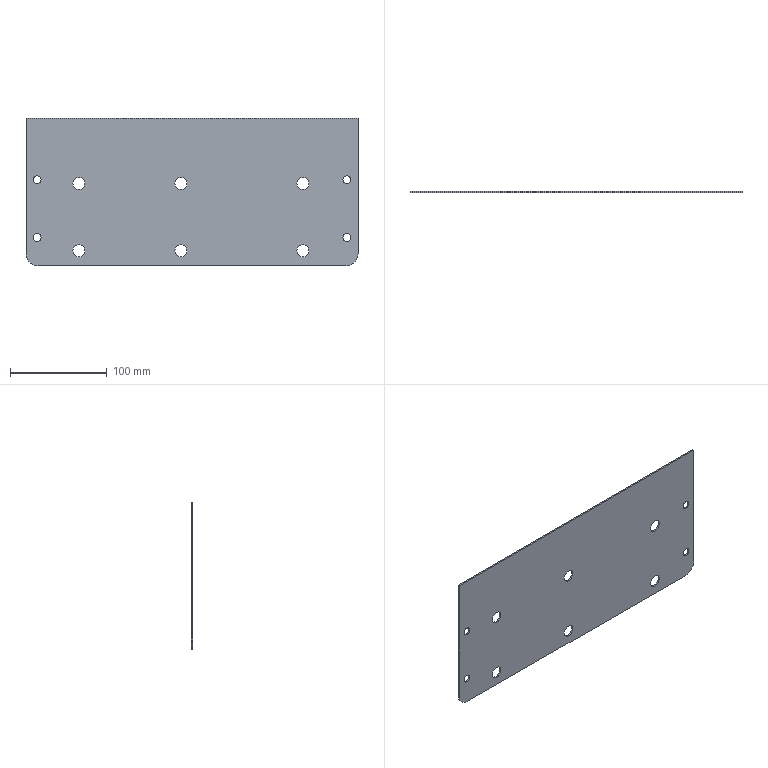Part | NX | features BREP 1 | 1 solid | 28 faces | box 342.9 x 1.499 x 152.4 mm | volume 76805 mm3 | cylinder 22 | plane 6 | commonest cylinder face diameters 12.446 x12 8.128 x8 25.4 x2
STEP:
#1=CARTESIAN_POINT('',(158.75,0.,-152.4));
#2=VERTEX_POINT('',#1);
#3=CARTESIAN_POINT('',(-158.75,0.,-152.4));
#4=VERTEX_POINT('',#3);
#5=CARTESIAN_POINT('',(158.75,0.,-152.4));
#6=DIRECTION('',(-1.,0.,0.));
#7=VECTOR('',#6,1000.);
#8=LINE('',#5,#7);
#9=EDGE_CURVE('',#2,#4,#8,.T.);
#10=ORIENTED_EDGE('',*,*,#9,.T.);
#11=CARTESIAN_POINT('',(-171.45,0.,-139.7));
#12=VERTEX_POINT('',#11);
#13=CARTESIAN_POINT('',(-158.75,0.,-139.7));
#14=DIRECTION('',(0.,1.,0.));
#15=DIRECTION('',(0.,0.,-1.));
#16=AXIS2_PLACEMENT_3D('',#13,#14,#15);
#17=CIRCLE('',#16,12.7);
#18=EDGE_CURVE('',#4,#12,#17,.T.);
#19=ORIENTED_EDGE('',*,*,#18,.T.);
#20=CARTESIAN_POINT('',(-171.45,0.,0.));
#21=VERTEX_POINT('',#20);
#22=CARTESIAN_POINT('',(-171.45,0.,-139.7));
#23=DIRECTION('',(0.,0.,1.));
#24=VECTOR('',#23,1000.);
#25=LINE('',#22,#24);
#26=EDGE_CURVE('',#12,#21,#25,.T.);
#27=ORIENTED_EDGE('',*,*,#26,.T.);
#28=CARTESIAN_POINT('',(171.45,0.,0.));
#29=VERTEX_POINT('',#28);
#30=CARTESIAN_POINT('',(-171.45,0.,0.));
#31=DIRECTION('',(1.,0.,0.));
#32=VECTOR('',#31,1000.);
#33=LINE('',#30,#32);
#34=EDGE_CURVE('',#21,#29,#33,.T.);
#35=ORIENTED_EDGE('',*,*,#34,.T.);
#36=CARTESIAN_POINT('',(171.45,0.,-139.7));
#37=VERTEX_POINT('',#36);
#38=CARTESIAN_POINT('',(171.45,0.,0.));
#39=DIRECTION('',(0.,0.,-1.));
#40=VECTOR('',#39,1000.);
#41=LINE('',#38,#40);
#42=EDGE_CURVE('',#29,#37,#41,.T.);
#43=ORIENTED_EDGE('',*,*,#42,.T.);
#44=CARTESIAN_POINT('',(158.75,0.,-139.7));
#45=DIRECTION('',(0.,1.,0.));
#46=DIRECTION('',(1.,0.,0.));
#47=AXIS2_PLACEMENT_3D('',#44,#45,#46);
#48=CIRCLE('',#47,12.7);
#49=EDGE_CURVE('',#37,#2,#48,.T.);
#50=ORIENTED_EDGE('',*,*,#49,.T.);
#51=EDGE_LOOP('',(#10,#19,#27,#35,#43,#50));
#52=FACE_BOUND('',#51,.T.);
#53=CARTESIAN_POINT('',(164.084,0.,-123.19));
#54=VERTEX_POINT('',#53);
#55=CARTESIAN_POINT('',(155.956,0.,-123.19));
#56=VERTEX_POINT('',#55);
#57=CARTESIAN_POINT('',(160.02,0.,-123.19));
#58=DIRECTION('',(0.,1.,0.));
#59=DIRECTION('',(1.,0.,0.));
#60=AXIS2_PLACEMENT_3D('',#57,#58,#59);
#61=CIRCLE('',#60,4.064);
#62=EDGE_CURVE('',#54,#56,#61,.T.);
#63=ORIENTED_EDGE('',*,*,#62,.F.);
#64=CARTESIAN_POINT('',(160.02,0.,-123.19));
#65=DIRECTION('',(0.,1.,0.));
#66=DIRECTION('',(-1.,0.,0.));
#67=AXIS2_PLACEMENT_3D('',#64,#65,#66);
#68=CIRCLE('',#67,4.064);
#69=EDGE_CURVE('',#56,#54,#68,.T.);
#70=ORIENTED_EDGE('',*,*,#69,.F.);
#71=EDGE_LOOP('',(#63,#70));
#72=FACE_BOUND('',#71,.T.);
#73=CARTESIAN_POINT('',(-164.084,0.,-63.5));
#74=VERTEX_POINT('',#73);
#75=CARTESIAN_POINT('',(-155.956,0.,-63.5));
#76=VERTEX_POINT('',#75);
#77=CARTESIAN_POINT('',(-160.02,0.,-63.5));
#78=DIRECTION('',(0.,-1.,0.));
#79=DIRECTION('',(-1.,0.,0.));
#80=AXIS2_PLACEMENT_3D('',#77,#78,#79);
#81=CIRCLE('',#80,4.064);
#82=EDGE_CURVE('',#74,#76,#81,.T.);
#83=ORIENTED_EDGE('',*,*,#82,.T.);
#84=CARTESIAN_POINT('',(-160.02,0.,-63.5));
#85=DIRECTION('',(0.,-1.,0.));
#86=DIRECTION('',(1.,0.,0.));
#87=AXIS2_PLACEMENT_3D('',#84,#85,#86);
#88=CIRCLE('',#87,4.064);
#89=EDGE_CURVE('',#76,#74,#88,.T.);
#90=ORIENTED_EDGE('',*,*,#89,.T.);
#91=EDGE_LOOP('',(#83,#90));
#92=FACE_BOUND('',#91,.T.);
#93=CARTESIAN_POINT('',(-164.084,0.,-123.19));
#94=VERTEX_POINT('',#93);
#95=CARTESIAN_POINT('',(-155.956,0.,-123.19));
#96=VERTEX_POINT('',#95);
#97=CARTESIAN_POINT('',(-160.02,0.,-123.19));
#98=DIRECTION('',(0.,-1.,0.));
#99=DIRECTION('',(-1.,0.,0.));
#100=AXIS2_PLACEMENT_3D('',#97,#98,#99);
#101=CIRCLE('',#100,4.064);
#102=EDGE_CURVE('',#94,#96,#101,.T.);
#103=ORIENTED_EDGE('',*,*,#102,.T.);
#104=CARTESIAN_POINT('',(-160.02,0.,-123.19));
#105=DIRECTION('',(0.,-1.,0.));
#106=DIRECTION('',(1.,0.,0.));
#107=AXIS2_PLACEMENT_3D('',#104,#105,#106);
#108=CIRCLE('',#107,4.064);
#109=EDGE_CURVE('',#96,#94,#108,.T.);
#110=ORIENTED_EDGE('',*,*,#109,.T.);
#111=EDGE_LOOP('',(#103,#110));
#112=FACE_BOUND('',#111,.T.);
#113=CARTESIAN_POINT('',(164.084,0.,-63.5));
#114=VERTEX_POINT('',#113);
#115=CARTESIAN_POINT('',(155.956,0.,-63.5));
#116=VERTEX_POINT('',#115);
#117=CARTESIAN_POINT('',(160.02,0.,-63.5));
#118=DIRECTION('',(0.,1.,0.));
#119=DIRECTION('',(1.,0.,0.));
#120=AXIS2_PLACEMENT_3D('',#117,#118,#119);
#121=CIRCLE('',#120,4.064);
#122=EDGE_CURVE('',#114,#116,#121,.T.);
#123=ORIENTED_EDGE('',*,*,#122,.F.);
#124=CARTESIAN_POINT('',(160.02,0.,-63.5));
#125=DIRECTION('',(0.,1.,0.));
#126=DIRECTION('',(-1.,0.,0.));
#127=AXIS2_PLACEMENT_3D('',#124,#125,#126);
#128=CIRCLE('',#127,4.064);
#129=EDGE_CURVE('',#116,#114,#128,.T.);
#130=ORIENTED_EDGE('',*,*,#129,.F.);
#131=EDGE_LOOP('',(#123,#130));
#132=FACE_BOUND('',#131,.T.);
#133=CARTESIAN_POINT('',(108.331,0.,-67.31));
#134=VERTEX_POINT('',#133);
#135=CARTESIAN_POINT('',(120.777,0.,-67.31));
#136=VERTEX_POINT('',#135);
#137=CARTESIAN_POINT('',(114.554,0.,-67.31));
#138=DIRECTION('',(0.,1.,0.));
#139=DIRECTION('',(-1.,0.,0.));
#140=AXIS2_PLACEMENT_3D('',#137,#138,#139);
#141=CIRCLE('',#140,6.223);
#142=EDGE_CURVE('',#134,#136,#141,.T.);
#143=ORIENTED_EDGE('',*,*,#142,.F.);
#144=CARTESIAN_POINT('',(114.554,0.,-67.31));
#145=DIRECTION('',(0.,1.,0.));
#146=DIRECTION('',(1.,0.,0.));
#147=AXIS2_PLACEMENT_3D('',#144,#145,#146);
#148=CIRCLE('',#147,6.223);
#149=EDGE_CURVE('',#136,#134,#148,.T.);
#150=ORIENTED_EDGE('',*,*,#149,.F.);
#151=EDGE_LOOP('',(#143,#150));
#152=FACE_BOUND('',#151,.T.);
#153=CARTESIAN_POINT('',(-17.653,0.,-67.31));
#154=VERTEX_POINT('',#153);
#155=CARTESIAN_POINT('',(-5.207,0.,-67.31));
#156=VERTEX_POINT('',#155);
#157=CARTESIAN_POINT('',(-11.43,0.,-67.31));
#158=DIRECTION('',(0.,1.,0.));
#159=DIRECTION('',(-1.,0.,0.));
#160=AXIS2_PLACEMENT_3D('',#157,#158,#159);
#161=CIRCLE('',#160,6.223);
#162=EDGE_CURVE('',#154,#156,#161,.T.);
#163=ORIENTED_EDGE('',*,*,#162,.F.);
#164=CARTESIAN_POINT('',(-11.43,0.,-67.31));
#165=DIRECTION('',(0.,1.,0.));
#166=DIRECTION('',(1.,0.,0.));
#167=AXIS2_PLACEMENT_3D('',#164,#165,#166);
#168=CIRCLE('',#167,6.223);
#169=EDGE_CURVE('',#156,#154,#168,.T.);
#170=ORIENTED_EDGE('',*,*,#169,.F.);
#171=EDGE_LOOP('',(#163,#170));
#172=FACE_BOUND('',#171,.T.);
#173=CARTESIAN_POINT('',(-123.063,0.,-67.31));
#174=VERTEX_POINT('',#173);
#175=CARTESIAN_POINT('',(-110.617,0.,-67.31));
#176=VERTEX_POINT('',#175);
#177=CARTESIAN_POINT('',(-116.84,0.,-67.31));
#178=DIRECTION('',(0.,1.,0.));
#179=DIRECTION('',(-1.,0.,0.));
#180=AXIS2_PLACEMENT_3D('',#177,#178,#179);
#181=CIRCLE('',#180,6.223);
#182=EDGE_CURVE('',#174,#176,#181,.T.);
#183=ORIENTED_EDGE('',*,*,#182,.F.);
#184=CARTESIAN_POINT('',(-116.84,0.,-67.31));
#185=DIRECTION('',(0.,1.,0.));
#186=DIRECTION('',(1.,0.,0.));
#187=AXIS2_PLACEMENT_3D('',#184,#185,#186);
#188=CIRCLE('',#187,6.223);
#189=EDGE_CURVE('',#176,#174,#188,.T.);
#190=ORIENTED_EDGE('',*,*,#189,.F.);
#191=EDGE_LOOP('',(#183,#190));
#192=FACE_BOUND('',#191,.T.);
#193=CARTESIAN_POINT('',(-17.653,0.,-136.906));
#194=VERTEX_POINT('',#193);
#195=CARTESIAN_POINT('',(-5.207,0.,-136.906));
#196=VERTEX_POINT('',#195);
#197=CARTESIAN_POINT('',(-11.43,0.,-136.906));
#198=DIRECTION('',(0.,1.,0.));
#199=DIRECTION('',(-1.,0.,0.));
#200=AXIS2_PLACEMENT_3D('',#197,#198,#199);
#201=CIRCLE('',#200,6.223);
#202=EDGE_CURVE('',#194,#196,#201,.T.);
#203=ORIENTED_EDGE('',*,*,#202,.F.);
#204=CARTESIAN_POINT('',(-11.43,0.,-136.906));
#205=DIRECTION('',(0.,1.,0.));
#206=DIRECTION('',(1.,0.,0.));
#207=AXIS2_PLACEMENT_3D('',#204,#205,#206);
#208=CIRCLE('',#207,6.223);
#209=EDGE_CURVE('',#196,#194,#208,.T.);
#210=ORIENTED_EDGE('',*,*,#209,.F.);
#211=EDGE_LOOP('',(#203,#210));
#212=FACE_BOUND('',#211,.T.);
#213=CARTESIAN_POINT('',(108.331,0.,-136.906));
#214=VERTEX_POINT('',#213);
#215=CARTESIAN_POINT('',(120.777,0.,-136.906));
#216=VERTEX_POINT('',#215);
#217=CARTESIAN_POINT('',(114.554,0.,-136.906));
#218=DIRECTION('',(0.,1.,0.));
#219=DIRECTION('',(-1.,0.,0.));
#220=AXIS2_PLACEMENT_3D('',#217,#218,#219);
#221=CIRCLE('',#220,6.223);
#222=EDGE_CURVE('',#214,#216,#221,.T.);
#223=ORIENTED_EDGE('',*,*,#222,.F.);
#224=CARTESIAN_POINT('',(114.554,0.,-136.906));
#225=DIRECTION('',(0.,1.,0.));
#226=DIRECTION('',(1.,0.,0.));
#227=AXIS2_PLACEMENT_3D('',#224,#225,#226);
#228=CIRCLE('',#227,6.223);
#229=EDGE_CURVE('',#216,#214,#228,.T.);
#230=ORIENTED_EDGE('',*,*,#229,.F.);
#231=EDGE_LOOP('',(#223,#230));
#232=FACE_BOUND('',#231,.T.);
#233=CARTESIAN_POINT('',(-123.063,0.,-136.906));
#234=VERTEX_POINT('',#233);
#235=CARTESIAN_POINT('',(-110.617,0.,-136.906));
#236=VERTEX_POINT('',#235);
#237=CARTESIAN_POINT('',(-116.84,0.,-136.906));
#238=DIRECTION('',(0.,1.,0.));
#239=DIRECTION('',(-1.,0.,0.));
#240=AXIS2_PLACEMENT_3D('',#237,#238,#239);
#241=CIRCLE('',#240,6.223);
#242=EDGE_CURVE('',#234,#236,#241,.T.);
#243=ORIENTED_EDGE('',*,*,#242,.F.);
#244=CARTESIAN_POINT('',(-116.84,0.,-136.906));
#245=DIRECTION('',(0.,1.,0.));
#246=DIRECTION('',(1.,0.,0.));
#247=AXIS2_PLACEMENT_3D('',#244,#245,#246);
#248=CIRCLE('',#247,6.223);
#249=EDGE_CURVE('',#236,#234,#248,.T.);
#250=ORIENTED_EDGE('',*,*,#249,.F.);
#251=EDGE_LOOP('',(#243,#250));
#252=FACE_BOUND('',#251,.T.);
#253=CARTESIAN_POINT('',(0.,0.,0.));
#254=DIRECTION('',(0.,1.,0.));
#255=DIRECTION('',(1.,0.,0.));
#256=AXIS2_PLACEMENT_3D('',#253,#254,#255);
#257=PLANE('',#256);
#258=ADVANCED_FACE('',(#52,#72,#92,#112,#132,#152,#172,#192,#212,#232,#252),#257,.T.);
#259=CARTESIAN_POINT('',(164.084,-1.499,-63.5));
#260=VERTEX_POINT('',#259);
#261=CARTESIAN_POINT('',(164.084,0.,-63.5));
#262=DIRECTION('',(0.,-1.,0.));
#263=VECTOR('',#262,1000.);
#264=LINE('',#261,#263);
#265=EDGE_CURVE('',#260,#114,#264,.F.);
#266=ORIENTED_EDGE('',*,*,#265,.F.);
#267=CARTESIAN_POINT('',(155.956,-1.499,-63.5));
#268=VERTEX_POINT('',#267);
#269=CARTESIAN_POINT('',(160.02,-1.499,-63.5));
#270=DIRECTION('',(0.,1.,0.));
#271=DIRECTION('',(-1.,0.,0.));
#272=AXIS2_PLACEMENT_3D('',#269,#270,#271);
#273=CIRCLE('',#272,4.064);
#274=EDGE_CURVE('',#268,#260,#273,.T.);
#275=ORIENTED_EDGE('',*,*,#274,.F.);
#276=CARTESIAN_POINT('',(155.956,0.,-63.5));
#277=DIRECTION('',(0.,-1.,0.));
#278=VECTOR('',#277,1000.);
#279=LINE('',#276,#278);
#280=EDGE_CURVE('',#268,#116,#279,.F.);
#281=ORIENTED_EDGE('',*,*,#280,.T.);
#282=ORIENTED_EDGE('',*,*,#129,.T.);
#283=EDGE_LOOP('',(#266,#275,#281,#282));
#284=FACE_BOUND('',#283,.T.);
#285=CARTESIAN_POINT('',(160.02,-0.7493,-63.5));
#286=DIRECTION('',(0.,1.,0.));
#287=DIRECTION('',(-1.,0.,0.));
#288=AXIS2_PLACEMENT_3D('',#285,#286,#287);
#289=CYLINDRICAL_SURFACE('',#288,4.064);
#290=ADVANCED_FACE('',(#284),#289,.F.);
#291=ORIENTED_EDGE('',*,*,#280,.F.);
#292=CARTESIAN_POINT('',(160.02,-1.499,-63.5));
#293=DIRECTION('',(0.,1.,0.));
#294=DIRECTION('',(1.,0.,0.));
#295=AXIS2_PLACEMENT_3D('',#292,#293,#294);
#296=CIRCLE('',#295,4.064);
#297=EDGE_CURVE('',#260,#268,#296,.T.);
#298=ORIENTED_EDGE('',*,*,#297,.F.);
#299=ORIENTED_EDGE('',*,*,#265,.T.);
#300=ORIENTED_EDGE('',*,*,#122,.T.);
#301=EDGE_LOOP('',(#291,#298,#299,#300));
#302=FACE_BOUND('',#301,.T.);
#303=CARTESIAN_POINT('',(160.02,-0.7493,-63.5));
#304=DIRECTION('',(0.,1.,0.));
#305=DIRECTION('',(1.,0.,0.));
#306=AXIS2_PLACEMENT_3D('',#303,#304,#305);
#307=CYLINDRICAL_SURFACE('',#306,4.064);
#308=ADVANCED_FACE('',(#302),#307,.F.);
#309=CARTESIAN_POINT('',(171.45,-1.499,0.));
#310=VERTEX_POINT('',#309);
#311=CARTESIAN_POINT('',(171.45,-1.499,-139.7));
#312=VERTEX_POINT('',#311);
#313=CARTESIAN_POINT('',(171.45,-1.499,0.));
#314=DIRECTION('',(0.,0.,-1.));
#315=VECTOR('',#314,1000.);
#316=LINE('',#313,#315);
#317=EDGE_CURVE('',#310,#312,#316,.T.);
#318=ORIENTED_EDGE('',*,*,#317,.F.);
#319=CARTESIAN_POINT('',(-171.45,-1.499,0.));
#320=VERTEX_POINT('',#319);
#321=CARTESIAN_POINT('',(-171.45,-1.499,0.));
#322=DIRECTION('',(1.,0.,0.));
#323=VECTOR('',#322,1000.);
#324=LINE('',#321,#323);
#325=EDGE_CURVE('',#320,#310,#324,.T.);
#326=ORIENTED_EDGE('',*,*,#325,.F.);
#327=CARTESIAN_POINT('',(-171.45,-1.499,-139.7));
#328=VERTEX_POINT('',#327);
#329=CARTESIAN_POINT('',(-171.45,-1.499,-139.7));
#330=DIRECTION('',(0.,0.,1.));
#331=VECTOR('',#330,1000.);
#332=LINE('',#329,#331);
#333=EDGE_CURVE('',#328,#320,#332,.T.);
#334=ORIENTED_EDGE('',*,*,#333,.F.);
#335=CARTESIAN_POINT('',(-158.75,-1.499,-152.4));
#336=VERTEX_POINT('',#335);
#337=CARTESIAN_POINT('',(-158.75,-1.499,-139.7));
#338=DIRECTION('',(0.,-1.,0.));
#339=DIRECTION('',(-1.,0.,0.));
#340=AXIS2_PLACEMENT_3D('',#337,#338,#339);
#341=CIRCLE('',#340,12.7);
#342=EDGE_CURVE('',#328,#336,#341,.T.);
#343=ORIENTED_EDGE('',*,*,#342,.T.);
#344=CARTESIAN_POINT('',(158.75,-1.499,-152.4));
#345=VERTEX_POINT('',#344);
#346=CARTESIAN_POINT('',(158.75,-1.499,-152.4));
#347=DIRECTION('',(-1.,0.,0.));
#348=VECTOR('',#347,1000.);
#349=LINE('',#346,#348);
#350=EDGE_CURVE('',#345,#336,#349,.T.);
#351=ORIENTED_EDGE('',*,*,#350,.F.);
#352=CARTESIAN_POINT('',(158.75,-1.499,-139.7));
#353=DIRECTION('',(0.,-1.,0.));
#354=DIRECTION('',(0.,0.,-1.));
#355=AXIS2_PLACEMENT_3D('',#352,#353,#354);
#356=CIRCLE('',#355,12.7);
#357=EDGE_CURVE('',#345,#312,#356,.T.);
#358=ORIENTED_EDGE('',*,*,#357,.T.);
#359=EDGE_LOOP('',(#318,#326,#334,#343,#351,#358));
#360=FACE_BOUND('',#359,.T.);
#361=ORIENTED_EDGE('',*,*,#297,.T.);
#362=ORIENTED_EDGE('',*,*,#274,.T.);
#363=EDGE_LOOP('',(#361,#362));
#364=FACE_BOUND('',#363,.T.);
#365=CARTESIAN_POINT('',(-164.084,-1.499,-123.19));
#366=VERTEX_POINT('',#365);
#367=CARTESIAN_POINT('',(-155.956,-1.499,-123.19));
#368=VERTEX_POINT('',#367);
#369=CARTESIAN_POINT('',(-160.02,-1.499,-123.19));
#370=DIRECTION('',(0.,-1.,0.));
#371=DIRECTION('',(-1.,0.,0.));
#372=AXIS2_PLACEMENT_3D('',#369,#370,#371);
#373=CIRCLE('',#372,4.064);
#374=EDGE_CURVE('',#366,#368,#373,.T.);
#375=ORIENTED_EDGE('',*,*,#374,.F.);
#376=CARTESIAN_POINT('',(-160.02,-1.499,-123.19));
#377=DIRECTION('',(0.,-1.,0.));
#378=DIRECTION('',(1.,0.,0.));
#379=AXIS2_PLACEMENT_3D('',#376,#377,#378);
#380=CIRCLE('',#379,4.064);
#381=EDGE_CURVE('',#368,#366,#380,.T.);
#382=ORIENTED_EDGE('',*,*,#381,.F.);
#383=EDGE_LOOP('',(#375,#382));
#384=FACE_BOUND('',#383,.T.);
#385=CARTESIAN_POINT('',(-164.084,-1.499,-63.5));
#386=VERTEX_POINT('',#385);
#387=CARTESIAN_POINT('',(-155.956,-1.499,-63.5));
#388=VERTEX_POINT('',#387);
#389=CARTESIAN_POINT('',(-160.02,-1.499,-63.5));
#390=DIRECTION('',(0.,-1.,0.));
#391=DIRECTION('',(-1.,0.,0.));
#392=AXIS2_PLACEMENT_3D('',#389,#390,#391);
#393=CIRCLE('',#392,4.064);
#394=EDGE_CURVE('',#386,#388,#393,.T.);
#395=ORIENTED_EDGE('',*,*,#394,.F.);
#396=CARTESIAN_POINT('',(-160.02,-1.499,-63.5));
#397=DIRECTION('',(0.,-1.,0.));
#398=DIRECTION('',(1.,0.,0.));
#399=AXIS2_PLACEMENT_3D('',#396,#397,#398);
#400=CIRCLE('',#399,4.064);
#401=EDGE_CURVE('',#388,#386,#400,.T.);
#402=ORIENTED_EDGE('',*,*,#401,.F.);
#403=EDGE_LOOP('',(#395,#402));
#404=FACE_BOUND('',#403,.T.);
#405=CARTESIAN_POINT('',(164.084,-1.499,-123.19));
#406=VERTEX_POINT('',#405);
#407=CARTESIAN_POINT('',(155.956,-1.499,-123.19));
#408=VERTEX_POINT('',#407);
#409=CARTESIAN_POINT('',(160.02,-1.499,-123.19));
#410=DIRECTION('',(0.,1.,0.));
#411=DIRECTION('',(1.,0.,0.));
#412=AXIS2_PLACEMENT_3D('',#409,#410,#411);
#413=CIRCLE('',#412,4.064);
#414=EDGE_CURVE('',#406,#408,#413,.T.);
#415=ORIENTED_EDGE('',*,*,#414,.T.);
#416=CARTESIAN_POINT('',(160.02,-1.499,-123.19));
#417=DIRECTION('',(0.,1.,0.));
#418=DIRECTION('',(-1.,0.,0.));
#419=AXIS2_PLACEMENT_3D('',#416,#417,#418);
#420=CIRCLE('',#419,4.064);
#421=EDGE_CURVE('',#408,#406,#420,.T.);
#422=ORIENTED_EDGE('',*,*,#421,.T.);
#423=EDGE_LOOP('',(#415,#422));
#424=FACE_BOUND('',#423,.T.);
#425=CARTESIAN_POINT('',(-123.063,-1.499,-136.906));
#426=VERTEX_POINT('',#425);
#427=CARTESIAN_POINT('',(-110.617,-1.499,-136.906));
#428=VERTEX_POINT('',#427);
#429=CARTESIAN_POINT('',(-116.84,-1.499,-136.906));
#430=DIRECTION('',(0.,1.,0.));
#431=DIRECTION('',(-1.,0.,0.));
#432=AXIS2_PLACEMENT_3D('',#429,#430,#431);
#433=CIRCLE('',#432,6.223);
#434=EDGE_CURVE('',#426,#428,#433,.T.);
#435=ORIENTED_EDGE('',*,*,#434,.T.);
#436=CARTESIAN_POINT('',(-116.84,-1.499,-136.906));
#437=DIRECTION('',(0.,1.,0.));
#438=DIRECTION('',(1.,0.,0.));
#439=AXIS2_PLACEMENT_3D('',#436,#437,#438);
#440=CIRCLE('',#439,6.223);
#441=EDGE_CURVE('',#428,#426,#440,.T.);
#442=ORIENTED_EDGE('',*,*,#441,.T.);
#443=EDGE_LOOP('',(#435,#442));
#444=FACE_BOUND('',#443,.T.);
#445=CARTESIAN_POINT('',(108.331,-1.499,-136.906));
#446=VERTEX_POINT('',#445);
#447=CARTESIAN_POINT('',(120.777,-1.499,-136.906));
#448=VERTEX_POINT('',#447);
#449=CARTESIAN_POINT('',(114.554,-1.499,-136.906));
#450=DIRECTION('',(0.,1.,0.));
#451=DIRECTION('',(-1.,0.,0.));
#452=AXIS2_PLACEMENT_3D('',#449,#450,#451);
#453=CIRCLE('',#452,6.223);
#454=EDGE_CURVE('',#446,#448,#453,.T.);
#455=ORIENTED_EDGE('',*,*,#454,.T.);
#456=CARTESIAN_POINT('',(114.554,-1.499,-136.906));
#457=DIRECTION('',(0.,1.,0.));
#458=DIRECTION('',(1.,0.,0.));
#459=AXIS2_PLACEMENT_3D('',#456,#457,#458);
#460=CIRCLE('',#459,6.223);
#461=EDGE_CURVE('',#448,#446,#460,.T.);
#462=ORIENTED_EDGE('',*,*,#461,.T.);
#463=EDGE_LOOP('',(#455,#462));
#464=FACE_BOUND('',#463,.T.);
#465=CARTESIAN_POINT('',(-17.653,-1.499,-136.906));
#466=VERTEX_POINT('',#465);
#467=CARTESIAN_POINT('',(-5.207,-1.499,-136.906));
#468=VERTEX_POINT('',#467);
#469=CARTESIAN_POINT('',(-11.43,-1.499,-136.906));
#470=DIRECTION('',(0.,1.,0.));
#471=DIRECTION('',(-1.,0.,0.));
#472=AXIS2_PLACEMENT_3D('',#469,#470,#471);
#473=CIRCLE('',#472,6.223);
#474=EDGE_CURVE('',#466,#468,#473,.T.);
#475=ORIENTED_EDGE('',*,*,#474,.T.);
#476=CARTESIAN_POINT('',(-11.43,-1.499,-136.906));
#477=DIRECTION('',(0.,1.,0.));
#478=DIRECTION('',(1.,0.,0.));
#479=AXIS2_PLACEMENT_3D('',#476,#477,#478);
#480=CIRCLE('',#479,6.223);
#481=EDGE_CURVE('',#468,#466,#480,.T.);
#482=ORIENTED_EDGE('',*,*,#481,.T.);
#483=EDGE_LOOP('',(#475,#482));
#484=FACE_BOUND('',#483,.T.);
#485=CARTESIAN_POINT('',(-123.063,-1.499,-67.31));
#486=VERTEX_POINT('',#485);
#487=CARTESIAN_POINT('',(-110.617,-1.499,-67.31));
#488=VERTEX_POINT('',#487);
#489=CARTESIAN_POINT('',(-116.84,-1.499,-67.31));
#490=DIRECTION('',(0.,1.,0.));
#491=DIRECTION('',(-1.,0.,0.));
#492=AXIS2_PLACEMENT_3D('',#489,#490,#491);
#493=CIRCLE('',#492,6.223);
#494=EDGE_CURVE('',#486,#488,#493,.T.);
#495=ORIENTED_EDGE('',*,*,#494,.T.);
#496=CARTESIAN_POINT('',(-116.84,-1.499,-67.31));
#497=DIRECTION('',(0.,1.,0.));
#498=DIRECTION('',(1.,0.,0.));
#499=AXIS2_PLACEMENT_3D('',#496,#497,#498);
#500=CIRCLE('',#499,6.223);
#501=EDGE_CURVE('',#488,#486,#500,.T.);
#502=ORIENTED_EDGE('',*,*,#501,.T.);
#503=EDGE_LOOP('',(#495,#502));
#504=FACE_BOUND('',#503,.T.);
#505=CARTESIAN_POINT('',(-17.653,-1.499,-67.31));
#506=VERTEX_POINT('',#505);
#507=CARTESIAN_POINT('',(-5.207,-1.499,-67.31));
#508=VERTEX_POINT('',#507);
#509=CARTESIAN_POINT('',(-11.43,-1.499,-67.31));
#510=DIRECTION('',(0.,1.,0.));
#511=DIRECTION('',(-1.,0.,0.));
#512=AXIS2_PLACEMENT_3D('',#509,#510,#511);
#513=CIRCLE('',#512,6.223);
#514=EDGE_CURVE('',#506,#508,#513,.T.);
#515=ORIENTED_EDGE('',*,*,#514,.T.);
#516=CARTESIAN_POINT('',(-11.43,-1.499,-67.31));
#517=DIRECTION('',(0.,1.,0.));
#518=DIRECTION('',(1.,0.,0.));
#519=AXIS2_PLACEMENT_3D('',#516,#517,#518);
#520=CIRCLE('',#519,6.223);
#521=EDGE_CURVE('',#508,#506,#520,.T.);
#522=ORIENTED_EDGE('',*,*,#521,.T.);
#523=EDGE_LOOP('',(#515,#522));
#524=FACE_BOUND('',#523,.T.);
#525=CARTESIAN_POINT('',(108.331,-1.499,-67.31));
#526=VERTEX_POINT('',#525);
#527=CARTESIAN_POINT('',(120.777,-1.499,-67.31));
#528=VERTEX_POINT('',#527);
#529=CARTESIAN_POINT('',(114.554,-1.499,-67.31));
#530=DIRECTION('',(0.,1.,0.));
#531=DIRECTION('',(-1.,0.,0.));
#532=AXIS2_PLACEMENT_3D('',#529,#530,#531);
#533=CIRCLE('',#532,6.223);
#534=EDGE_CURVE('',#526,#528,#533,.T.);
#535=ORIENTED_EDGE('',*,*,#534,.T.);
#536=CARTESIAN_POINT('',(114.554,-1.499,-67.31));
#537=DIRECTION('',(0.,1.,0.));
#538=DIRECTION('',(1.,0.,0.));
#539=AXIS2_PLACEMENT_3D('',#536,#537,#538);
#540=CIRCLE('',#539,6.223);
#541=EDGE_CURVE('',#528,#526,#540,.T.);
#542=ORIENTED_EDGE('',*,*,#541,.T.);
#543=EDGE_LOOP('',(#535,#542));
#544=FACE_BOUND('',#543,.T.);
#545=CARTESIAN_POINT('',(0.,-1.499,0.));
#546=DIRECTION('',(0.,1.,0.));
#547=DIRECTION('',(1.,0.,0.));
#548=AXIS2_PLACEMENT_3D('',#545,#546,#547);
#549=PLANE('',#548);
#550=ADVANCED_FACE('',(#360,#364,#384,#404,#424,#444,#464,#484,#504,#524,#544),#549,.F.);
#551=CARTESIAN_POINT('',(164.084,0.,-123.19));
#552=DIRECTION('',(0.,-1.,0.));
#553=VECTOR('',#552,1000.);
#554=LINE('',#551,#553);
#555=EDGE_CURVE('',#406,#54,#554,.F.);
#556=ORIENTED_EDGE('',*,*,#555,.F.);
#557=ORIENTED_EDGE('',*,*,#421,.F.);
#558=CARTESIAN_POINT('',(155.956,0.,-123.19));
#559=DIRECTION('',(0.,-1.,0.));
#560=VECTOR('',#559,1000.);
#561=LINE('',#558,#560);
#562=EDGE_CURVE('',#408,#56,#561,.F.);
#563=ORIENTED_EDGE('',*,*,#562,.T.);
#564=ORIENTED_EDGE('',*,*,#69,.T.);
#565=EDGE_LOOP('',(#556,#557,#563,#564));
#566=FACE_BOUND('',#565,.T.);
#567=CARTESIAN_POINT('',(160.02,-0.7493,-123.19));
#568=DIRECTION('',(0.,1.,0.));
#569=DIRECTION('',(-1.,0.,0.));
#570=AXIS2_PLACEMENT_3D('',#567,#568,#569);
#571=CYLINDRICAL_SURFACE('',#570,4.064);
#572=ADVANCED_FACE('',(#566),#571,.F.);
#573=ORIENTED_EDGE('',*,*,#562,.F.);
#574=ORIENTED_EDGE('',*,*,#414,.F.);
#575=ORIENTED_EDGE('',*,*,#555,.T.);
#576=ORIENTED_EDGE('',*,*,#62,.T.);
#577=EDGE_LOOP('',(#573,#574,#575,#576));
#578=FACE_BOUND('',#577,.T.);
#579=CARTESIAN_POINT('',(160.02,-0.7493,-123.19));
#580=DIRECTION('',(0.,1.,0.));
#581=DIRECTION('',(1.,0.,0.));
#582=AXIS2_PLACEMENT_3D('',#579,#580,#581);
#583=CYLINDRICAL_SURFACE('',#582,4.064);
#584=ADVANCED_FACE('',(#578),#583,.F.);
#585=CARTESIAN_POINT('',(-155.956,0.,-123.19));
#586=DIRECTION('',(0.,-1.,0.));
#587=VECTOR('',#586,1000.);
#588=LINE('',#585,#587);
#589=EDGE_CURVE('',#368,#96,#588,.F.);
#590=ORIENTED_EDGE('',*,*,#589,.F.);
#591=ORIENTED_EDGE('',*,*,#381,.T.);
#592=CARTESIAN_POINT('',(-164.084,0.,-123.19));
#593=DIRECTION('',(0.,-1.,0.));
#594=VECTOR('',#593,1000.);
#595=LINE('',#592,#594);
#596=EDGE_CURVE('',#366,#94,#595,.F.);
#597=ORIENTED_EDGE('',*,*,#596,.T.);
#598=ORIENTED_EDGE('',*,*,#109,.F.);
#599=EDGE_LOOP('',(#590,#591,#597,#598));
#600=FACE_BOUND('',#599,.T.);
#601=CARTESIAN_POINT('',(-160.02,-0.7493,-123.19));
#602=DIRECTION('',(0.,-1.,0.));
#603=DIRECTION('',(1.,0.,0.));
#604=AXIS2_PLACEMENT_3D('',#601,#602,#603);
#605=CYLINDRICAL_SURFACE('',#604,4.064);
#606=ADVANCED_FACE('',(#600),#605,.F.);
#607=ORIENTED_EDGE('',*,*,#596,.F.);
#608=ORIENTED_EDGE('',*,*,#374,.T.);
#609=ORIENTED_EDGE('',*,*,#589,.T.);
#610=ORIENTED_EDGE('',*,*,#102,.F.);
#611=EDGE_LOOP('',(#607,#608,#609,#610));
#612=FACE_BOUND('',#611,.T.);
#613=CARTESIAN_POINT('',(-160.02,-0.7493,-123.19));
#614=DIRECTION('',(0.,-1.,0.));
#615=DIRECTION('',(-1.,0.,0.));
#616=AXIS2_PLACEMENT_3D('',#613,#614,#615);
#617=CYLINDRICAL_SURFACE('',#616,4.064);
#618=ADVANCED_FACE('',(#612),#617,.F.);
#619=CARTESIAN_POINT('',(-155.956,0.,-63.5));
#620=DIRECTION('',(0.,-1.,0.));
#621=VECTOR('',#620,1000.);
#622=LINE('',#619,#621);
#623=EDGE_CURVE('',#388,#76,#622,.F.);
#624=ORIENTED_EDGE('',*,*,#623,.F.);
#625=ORIENTED_EDGE('',*,*,#401,.T.);
#626=CARTESIAN_POINT('',(-164.084,0.,-63.5));
#627=DIRECTION('',(0.,-1.,0.));
#628=VECTOR('',#627,1000.);
#629=LINE('',#626,#628);
#630=EDGE_CURVE('',#386,#74,#629,.F.);
#631=ORIENTED_EDGE('',*,*,#630,.T.);
#632=ORIENTED_EDGE('',*,*,#89,.F.);
#633=EDGE_LOOP('',(#624,#625,#631,#632));
#634=FACE_BOUND('',#633,.T.);
#635=CARTESIAN_POINT('',(-160.02,-0.7493,-63.5));
#636=DIRECTION('',(0.,-1.,0.));
#637=DIRECTION('',(1.,0.,0.));
#638=AXIS2_PLACEMENT_3D('',#635,#636,#637);
#639=CYLINDRICAL_SURFACE('',#638,4.064);
#640=ADVANCED_FACE('',(#634),#639,.F.);
#641=ORIENTED_EDGE('',*,*,#630,.F.);
#642=ORIENTED_EDGE('',*,*,#394,.T.);
#643=ORIENTED_EDGE('',*,*,#623,.T.);
#644=ORIENTED_EDGE('',*,*,#82,.F.);
#645=EDGE_LOOP('',(#641,#642,#643,#644));
#646=FACE_BOUND('',#645,.T.);
#647=CARTESIAN_POINT('',(-160.02,-0.7493,-63.5));
#648=DIRECTION('',(0.,-1.,0.));
#649=DIRECTION('',(-1.,0.,0.));
#650=AXIS2_PLACEMENT_3D('',#647,#648,#649);
#651=CYLINDRICAL_SURFACE('',#650,4.064);
#652=ADVANCED_FACE('',(#646),#651,.F.);
#653=ORIENTED_EDGE('',*,*,#357,.F.);
#654=CARTESIAN_POINT('',(158.75,-1.499,-152.4));
#655=DIRECTION('',(0.,1.,0.));
#656=VECTOR('',#655,1000.);
#657=LINE('',#654,#656);
#658=EDGE_CURVE('',#345,#2,#657,.T.);
#659=ORIENTED_EDGE('',*,*,#658,.T.);
#660=ORIENTED_EDGE('',*,*,#49,.F.);
#661=CARTESIAN_POINT('',(171.45,-1.499,-139.7));
#662=DIRECTION('',(0.,1.,0.));
#663=VECTOR('',#662,1000.);
#664=LINE('',#661,#663);
#665=EDGE_CURVE('',#312,#37,#664,.T.);
#666=ORIENTED_EDGE('',*,*,#665,.F.);
#667=EDGE_LOOP('',(#653,#659,#660,#666));
#668=FACE_BOUND('',#667,.T.);
#669=CARTESIAN_POINT('',(158.75,-2.009,-139.7));
#670=DIRECTION('',(0.,1.,0.));
#671=DIRECTION('',(1.,0.,0.));
#672=AXIS2_PLACEMENT_3D('',#669,#670,#671);
#673=CYLINDRICAL_SURFACE('',#672,12.7);
#674=ADVANCED_FACE('',(#668),#673,.T.);
#675=ORIENTED_EDGE('',*,*,#42,.F.);
#676=CARTESIAN_POINT('',(171.45,0.,0.));
#677=DIRECTION('',(0.,-1.,0.));
#678=VECTOR('',#677,1000.);
#679=LINE('',#676,#678);
#680=EDGE_CURVE('',#29,#310,#679,.T.);
#681=ORIENTED_EDGE('',*,*,#680,.T.);
#682=ORIENTED_EDGE('',*,*,#317,.T.);
#683=ORIENTED_EDGE('',*,*,#665,.T.);
#684=EDGE_LOOP('',(#675,#681,#682,#683));
#685=FACE_BOUND('',#684,.T.);
#686=CARTESIAN_POINT('',(171.45,-0.7493,-76.2));
#687=DIRECTION('',(1.,0.,0.));
#688=DIRECTION('',(0.,1.,0.));
#689=AXIS2_PLACEMENT_3D('',#686,#687,#688);
#690=PLANE('',#689);
#691=ADVANCED_FACE('',(#685),#690,.T.);
#692=CARTESIAN_POINT('',(-171.45,0.,0.));
#693=DIRECTION('',(0.,-1.,0.));
#694=VECTOR('',#693,1000.);
#695=LINE('',#692,#694);
#696=EDGE_CURVE('',#21,#320,#695,.T.);
#697=ORIENTED_EDGE('',*,*,#696,.T.);
#698=ORIENTED_EDGE('',*,*,#325,.T.);
#699=ORIENTED_EDGE('',*,*,#680,.F.);
#700=ORIENTED_EDGE('',*,*,#34,.F.);
#701=EDGE_LOOP('',(#697,#698,#699,#700));
#702=FACE_BOUND('',#701,.T.);
#703=CARTESIAN_POINT('',(0.,-0.7493,0.));
#704=DIRECTION('',(0.,0.,1.));
#705=DIRECTION('',(1.,0.,0.));
#706=AXIS2_PLACEMENT_3D('',#703,#704,#705);
#707=PLANE('',#706);
#708=ADVANCED_FACE('',(#702),#707,.T.);
#709=ORIENTED_EDGE('',*,*,#333,.T.);
#710=ORIENTED_EDGE('',*,*,#696,.F.);
#711=ORIENTED_EDGE('',*,*,#26,.F.);
#712=CARTESIAN_POINT('',(-171.45,-1.499,-139.7));
#713=DIRECTION('',(0.,1.,0.));
#714=VECTOR('',#713,1000.);
#715=LINE('',#712,#714);
#716=EDGE_CURVE('',#328,#12,#715,.T.);
#717=ORIENTED_EDGE('',*,*,#716,.F.);
#718=EDGE_LOOP('',(#709,#710,#711,#717));
#719=FACE_BOUND('',#718,.T.);
#720=CARTESIAN_POINT('',(-171.45,-0.7493,-76.2));
#721=DIRECTION('',(-1.,0.,0.));
#722=DIRECTION('',(0.,0.,1.));
#723=AXIS2_PLACEMENT_3D('',#720,#721,#722);
#724=PLANE('',#723);
#725=ADVANCED_FACE('',(#719),#724,.T.);
#726=ORIENTED_EDGE('',*,*,#342,.F.);
#727=ORIENTED_EDGE('',*,*,#716,.T.);
#728=ORIENTED_EDGE('',*,*,#18,.F.);
#729=CARTESIAN_POINT('',(-158.75,-1.499,-152.4));
#730=DIRECTION('',(0.,1.,0.));
#731=VECTOR('',#730,1000.);
#732=LINE('',#729,#731);
#733=EDGE_CURVE('',#336,#4,#732,.T.);
#734=ORIENTED_EDGE('',*,*,#733,.F.);
#735=EDGE_LOOP('',(#726,#727,#728,#734));
#736=FACE_BOUND('',#735,.T.);
#737=CARTESIAN_POINT('',(-158.75,-2.009,-139.7));
#738=DIRECTION('',(0.,1.,0.));
#739=DIRECTION('',(0.,0.,-1.));
#740=AXIS2_PLACEMENT_3D('',#737,#738,#739);
#741=CYLINDRICAL_SURFACE('',#740,12.7);
#742=ADVANCED_FACE('',(#736),#741,.T.);
#743=ORIENTED_EDGE('',*,*,#350,.T.);
#744=ORIENTED_EDGE('',*,*,#733,.T.);
#745=ORIENTED_EDGE('',*,*,#9,.F.);
#746=ORIENTED_EDGE('',*,*,#658,.F.);
#747=EDGE_LOOP('',(#743,#744,#745,#746));
#748=FACE_BOUND('',#747,.T.);
#749=CARTESIAN_POINT('',(0.,-0.7493,-152.4));
#750=DIRECTION('',(0.,0.,-1.));
#751=DIRECTION('',(0.,-1.,0.));
#752=AXIS2_PLACEMENT_3D('',#749,#750,#751);
#753=PLANE('',#752);
#754=ADVANCED_FACE('',(#748),#753,.T.);
#755=CARTESIAN_POINT('',(-123.063,0.,-136.906));
#756=DIRECTION('',(0.,-1.,0.));
#757=VECTOR('',#756,1000.);
#758=LINE('',#755,#757);
#759=EDGE_CURVE('',#234,#426,#758,.T.);
#760=ORIENTED_EDGE('',*,*,#759,.T.);
#761=ORIENTED_EDGE('',*,*,#441,.F.);
#762=CARTESIAN_POINT('',(-110.617,0.,-136.906));
#763=DIRECTION('',(0.,-1.,0.));
#764=VECTOR('',#763,1000.);
#765=LINE('',#762,#764);
#766=EDGE_CURVE('',#236,#428,#765,.T.);
#767=ORIENTED_EDGE('',*,*,#766,.F.);
#768=ORIENTED_EDGE('',*,*,#249,.T.);
#769=EDGE_LOOP('',(#760,#761,#767,#768));
#770=FACE_BOUND('',#769,.T.);
#771=CARTESIAN_POINT('',(-116.84,-0.7493,-136.906));
#772=DIRECTION('',(0.,1.,0.));
#773=DIRECTION('',(1.,0.,0.));
#774=AXIS2_PLACEMENT_3D('',#771,#772,#773);
#775=CYLINDRICAL_SURFACE('',#774,6.223);
#776=ADVANCED_FACE('',(#770),#775,.F.);
#777=ORIENTED_EDGE('',*,*,#766,.T.);
#778=ORIENTED_EDGE('',*,*,#434,.F.);
#779=ORIENTED_EDGE('',*,*,#759,.F.);
#780=ORIENTED_EDGE('',*,*,#242,.T.);
#781=EDGE_LOOP('',(#777,#778,#779,#780));
#782=FACE_BOUND('',#781,.T.);
#783=CARTESIAN_POINT('',(-116.84,-0.7493,-136.906));
#784=DIRECTION('',(0.,1.,0.));
#785=DIRECTION('',(-1.,0.,0.));
#786=AXIS2_PLACEMENT_3D('',#783,#784,#785);
#787=CYLINDRICAL_SURFACE('',#786,6.223);
#788=ADVANCED_FACE('',(#782),#787,.F.);
#789=CARTESIAN_POINT('',(108.331,0.,-136.906));
#790=DIRECTION('',(0.,-1.,0.));
#791=VECTOR('',#790,1000.);
#792=LINE('',#789,#791);
#793=EDGE_CURVE('',#214,#446,#792,.T.);
#794=ORIENTED_EDGE('',*,*,#793,.T.);
#795=ORIENTED_EDGE('',*,*,#461,.F.);
#796=CARTESIAN_POINT('',(120.777,0.,-136.906));
#797=DIRECTION('',(0.,-1.,0.));
#798=VECTOR('',#797,1000.);
#799=LINE('',#796,#798);
#800=EDGE_CURVE('',#216,#448,#799,.T.);
#801=ORIENTED_EDGE('',*,*,#800,.F.);
#802=ORIENTED_EDGE('',*,*,#229,.T.);
#803=EDGE_LOOP('',(#794,#795,#801,#802));
#804=FACE_BOUND('',#803,.T.);
#805=CARTESIAN_POINT('',(114.554,-0.7493,-136.906));
#806=DIRECTION('',(0.,1.,0.));
#807=DIRECTION('',(1.,0.,0.));
#808=AXIS2_PLACEMENT_3D('',#805,#806,#807);
#809=CYLINDRICAL_SURFACE('',#808,6.223);
#810=ADVANCED_FACE('',(#804),#809,.F.);
#811=ORIENTED_EDGE('',*,*,#800,.T.);
#812=ORIENTED_EDGE('',*,*,#454,.F.);
#813=ORIENTED_EDGE('',*,*,#793,.F.);
#814=ORIENTED_EDGE('',*,*,#222,.T.);
#815=EDGE_LOOP('',(#811,#812,#813,#814));
#816=FACE_BOUND('',#815,.T.);
#817=CARTESIAN_POINT('',(114.554,-0.7493,-136.906));
#818=DIRECTION('',(0.,1.,0.));
#819=DIRECTION('',(-1.,0.,0.));
#820=AXIS2_PLACEMENT_3D('',#817,#818,#819);
#821=CYLINDRICAL_SURFACE('',#820,6.223);
#822=ADVANCED_FACE('',(#816),#821,.F.);
#823=CARTESIAN_POINT('',(-17.653,0.,-136.906));
#824=DIRECTION('',(0.,-1.,0.));
#825=VECTOR('',#824,1000.);
#826=LINE('',#823,#825);
#827=EDGE_CURVE('',#194,#466,#826,.T.);
#828=ORIENTED_EDGE('',*,*,#827,.T.);
#829=ORIENTED_EDGE('',*,*,#481,.F.);
#830=CARTESIAN_POINT('',(-5.207,0.,-136.906));
#831=DIRECTION('',(0.,-1.,0.));
#832=VECTOR('',#831,1000.);
#833=LINE('',#830,#832);
#834=EDGE_CURVE('',#196,#468,#833,.T.);
#835=ORIENTED_EDGE('',*,*,#834,.F.);
#836=ORIENTED_EDGE('',*,*,#209,.T.);
#837=EDGE_LOOP('',(#828,#829,#835,#836));
#838=FACE_BOUND('',#837,.T.);
#839=CARTESIAN_POINT('',(-11.43,-0.7493,-136.906));
#840=DIRECTION('',(0.,1.,0.));
#841=DIRECTION('',(1.,0.,0.));
#842=AXIS2_PLACEMENT_3D('',#839,#840,#841);
#843=CYLINDRICAL_SURFACE('',#842,6.223);
#844=ADVANCED_FACE('',(#838),#843,.F.);
#845=ORIENTED_EDGE('',*,*,#834,.T.);
#846=ORIENTED_EDGE('',*,*,#474,.F.);
#847=ORIENTED_EDGE('',*,*,#827,.F.);
#848=ORIENTED_EDGE('',*,*,#202,.T.);
#849=EDGE_LOOP('',(#845,#846,#847,#848));
#850=FACE_BOUND('',#849,.T.);
#851=CARTESIAN_POINT('',(-11.43,-0.7493,-136.906));
#852=DIRECTION('',(0.,1.,0.));
#853=DIRECTION('',(-1.,0.,0.));
#854=AXIS2_PLACEMENT_3D('',#851,#852,#853);
#855=CYLINDRICAL_SURFACE('',#854,6.223);
#856=ADVANCED_FACE('',(#850),#855,.F.);
#857=CARTESIAN_POINT('',(-123.063,0.,-67.31));
#858=DIRECTION('',(0.,-1.,0.));
#859=VECTOR('',#858,1000.);
#860=LINE('',#857,#859);
#861=EDGE_CURVE('',#174,#486,#860,.T.);
#862=ORIENTED_EDGE('',*,*,#861,.T.);
#863=ORIENTED_EDGE('',*,*,#501,.F.);
#864=CARTESIAN_POINT('',(-110.617,0.,-67.31));
#865=DIRECTION('',(0.,-1.,0.));
#866=VECTOR('',#865,1000.);
#867=LINE('',#864,#866);
#868=EDGE_CURVE('',#176,#488,#867,.T.);
#869=ORIENTED_EDGE('',*,*,#868,.F.);
#870=ORIENTED_EDGE('',*,*,#189,.T.);
#871=EDGE_LOOP('',(#862,#863,#869,#870));
#872=FACE_BOUND('',#871,.T.);
#873=CARTESIAN_POINT('',(-116.84,-0.7493,-67.31));
#874=DIRECTION('',(0.,1.,0.));
#875=DIRECTION('',(1.,0.,0.));
#876=AXIS2_PLACEMENT_3D('',#873,#874,#875);
#877=CYLINDRICAL_SURFACE('',#876,6.223);
#878=ADVANCED_FACE('',(#872),#877,.F.);
#879=ORIENTED_EDGE('',*,*,#868,.T.);
#880=ORIENTED_EDGE('',*,*,#494,.F.);
#881=ORIENTED_EDGE('',*,*,#861,.F.);
#882=ORIENTED_EDGE('',*,*,#182,.T.);
#883=EDGE_LOOP('',(#879,#880,#881,#882));
#884=FACE_BOUND('',#883,.T.);
#885=CARTESIAN_POINT('',(-116.84,-0.7493,-67.31));
#886=DIRECTION('',(0.,1.,0.));
#887=DIRECTION('',(-1.,0.,0.));
#888=AXIS2_PLACEMENT_3D('',#885,#886,#887);
#889=CYLINDRICAL_SURFACE('',#888,6.223);
#890=ADVANCED_FACE('',(#884),#889,.F.);
#891=CARTESIAN_POINT('',(-17.653,0.,-67.31));
#892=DIRECTION('',(0.,-1.,0.));
#893=VECTOR('',#892,1000.);
#894=LINE('',#891,#893);
#895=EDGE_CURVE('',#154,#506,#894,.T.);
#896=ORIENTED_EDGE('',*,*,#895,.T.);
#897=ORIENTED_EDGE('',*,*,#521,.F.);
#898=CARTESIAN_POINT('',(-5.207,0.,-67.31));
#899=DIRECTION('',(0.,-1.,0.));
#900=VECTOR('',#899,1000.);
#901=LINE('',#898,#900);
#902=EDGE_CURVE('',#156,#508,#901,.T.);
#903=ORIENTED_EDGE('',*,*,#902,.F.);
#904=ORIENTED_EDGE('',*,*,#169,.T.);
#905=EDGE_LOOP('',(#896,#897,#903,#904));
#906=FACE_BOUND('',#905,.T.);
#907=CARTESIAN_POINT('',(-11.43,-0.7493,-67.31));
#908=DIRECTION('',(0.,1.,0.));
#909=DIRECTION('',(1.,0.,0.));
#910=AXIS2_PLACEMENT_3D('',#907,#908,#909);
#911=CYLINDRICAL_SURFACE('',#910,6.223);
#912=ADVANCED_FACE('',(#906),#911,.F.);
#913=ORIENTED_EDGE('',*,*,#902,.T.);
#914=ORIENTED_EDGE('',*,*,#514,.F.);
#915=ORIENTED_EDGE('',*,*,#895,.F.);
#916=ORIENTED_EDGE('',*,*,#162,.T.);
#917=EDGE_LOOP('',(#913,#914,#915,#916));
#918=FACE_BOUND('',#917,.T.);
#919=CARTESIAN_POINT('',(-11.43,-0.7493,-67.31));
#920=DIRECTION('',(0.,1.,0.));
#921=DIRECTION('',(-1.,0.,0.));
#922=AXIS2_PLACEMENT_3D('',#919,#920,#921);
#923=CYLINDRICAL_SURFACE('',#922,6.223);
#924=ADVANCED_FACE('',(#918),#923,.F.);
#925=CARTESIAN_POINT('',(108.331,0.,-67.31));
#926=DIRECTION('',(0.,-1.,0.));
#927=VECTOR('',#926,1000.);
#928=LINE('',#925,#927);
#929=EDGE_CURVE('',#134,#526,#928,.T.);
#930=ORIENTED_EDGE('',*,*,#929,.T.);
#931=ORIENTED_EDGE('',*,*,#541,.F.);
#932=CARTESIAN_POINT('',(120.777,0.,-67.31));
#933=DIRECTION('',(0.,-1.,0.));
#934=VECTOR('',#933,1000.);
#935=LINE('',#932,#934);
#936=EDGE_CURVE('',#136,#528,#935,.T.);
#937=ORIENTED_EDGE('',*,*,#936,.F.);
#938=ORIENTED_EDGE('',*,*,#149,.T.);
#939=EDGE_LOOP('',(#930,#931,#937,#938));
#940=FACE_BOUND('',#939,.T.);
#941=CARTESIAN_POINT('',(114.554,-0.7493,-67.31));
#942=DIRECTION('',(0.,1.,0.));
#943=DIRECTION('',(1.,0.,0.));
#944=AXIS2_PLACEMENT_3D('',#941,#942,#943);
#945=CYLINDRICAL_SURFACE('',#944,6.223);
#946=ADVANCED_FACE('',(#940),#945,.F.);
#947=ORIENTED_EDGE('',*,*,#936,.T.);
#948=ORIENTED_EDGE('',*,*,#534,.F.);
#949=ORIENTED_EDGE('',*,*,#929,.F.);
#950=ORIENTED_EDGE('',*,*,#142,.T.);
#951=EDGE_LOOP('',(#947,#948,#949,#950));
#952=FACE_BOUND('',#951,.T.);
#953=CARTESIAN_POINT('',(114.554,-0.7493,-67.31));
#954=DIRECTION('',(0.,1.,0.));
#955=DIRECTION('',(-1.,0.,0.));
#956=AXIS2_PLACEMENT_3D('',#953,#954,#955);
#957=CYLINDRICAL_SURFACE('',#956,6.223);
#958=ADVANCED_FACE('',(#952),#957,.F.);
#959=CLOSED_SHELL('',(#258,#290,#308,#550,#572,#584,#606,#618,#640,#652,#674,#691,#708,#725,#742,#754,#776,#788,#810,#822,#844,#856,#878,#890,#912,#924,#946,#958));
#960=MANIFOLD_SOLID_BREP('',#959);
#961=(LENGTH_UNIT()NAMED_UNIT(*)SI_UNIT(.MILLI.,.METRE.));
#962=UNCERTAINTY_MEASURE_WITH_UNIT(LENGTH_MEASURE(0.00001),#961,'','');
#963=(NAMED_UNIT(*)PLANE_ANGLE_UNIT()SI_UNIT($,.RADIAN.));
#964=(NAMED_UNIT(*)SI_UNIT($,.STERADIAN.)SOLID_ANGLE_UNIT());
#965=(GEOMETRIC_REPRESENTATION_CONTEXT(3)GLOBAL_UNCERTAINTY_ASSIGNED_CONTEXT((#962))GLOBAL_UNIT_ASSIGNED_CONTEXT((#961,#963,#964))REPRESENTATION_CONTEXT('',''));
#966=ADVANCED_BREP_SHAPE_REPRESENTATION('',(#960),#965);